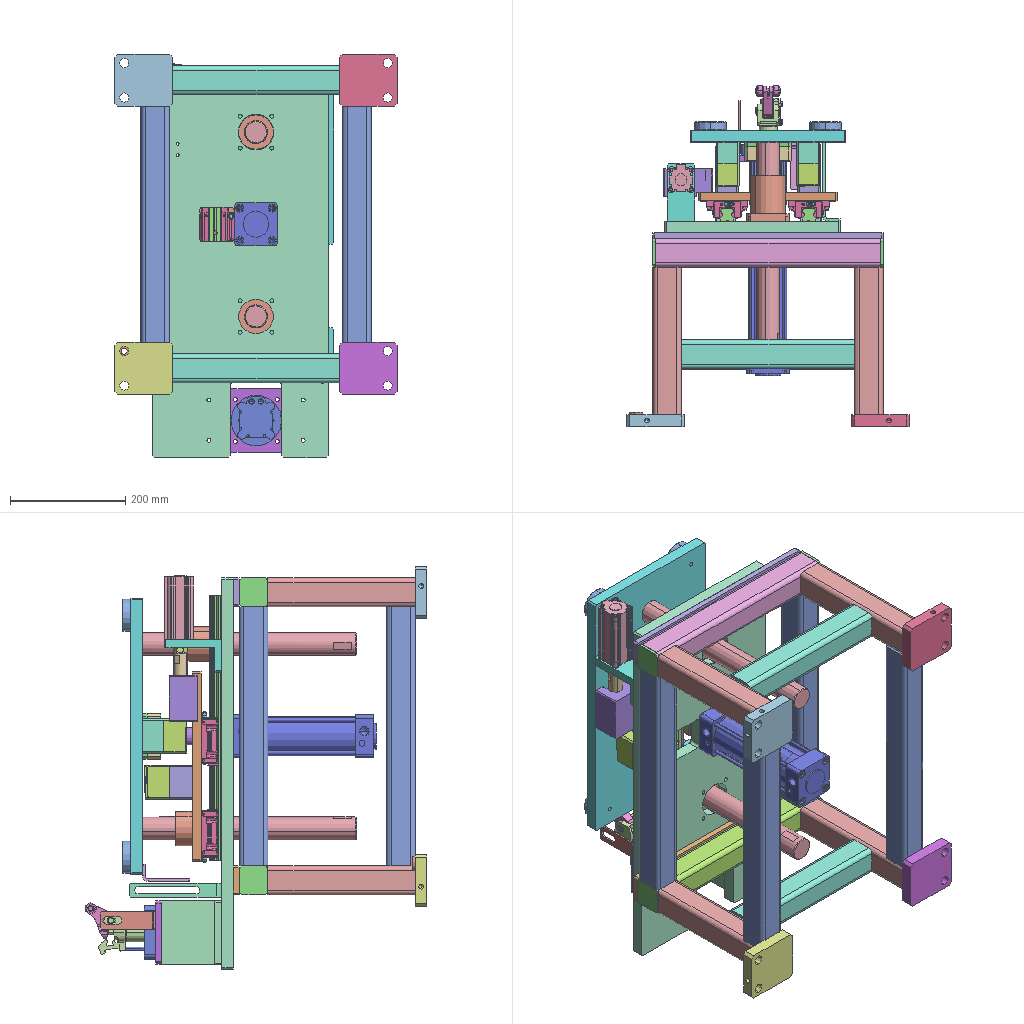Assembly | SolidWorks | 54 different items | 89 placed | box 490 x 593 x 700 mm
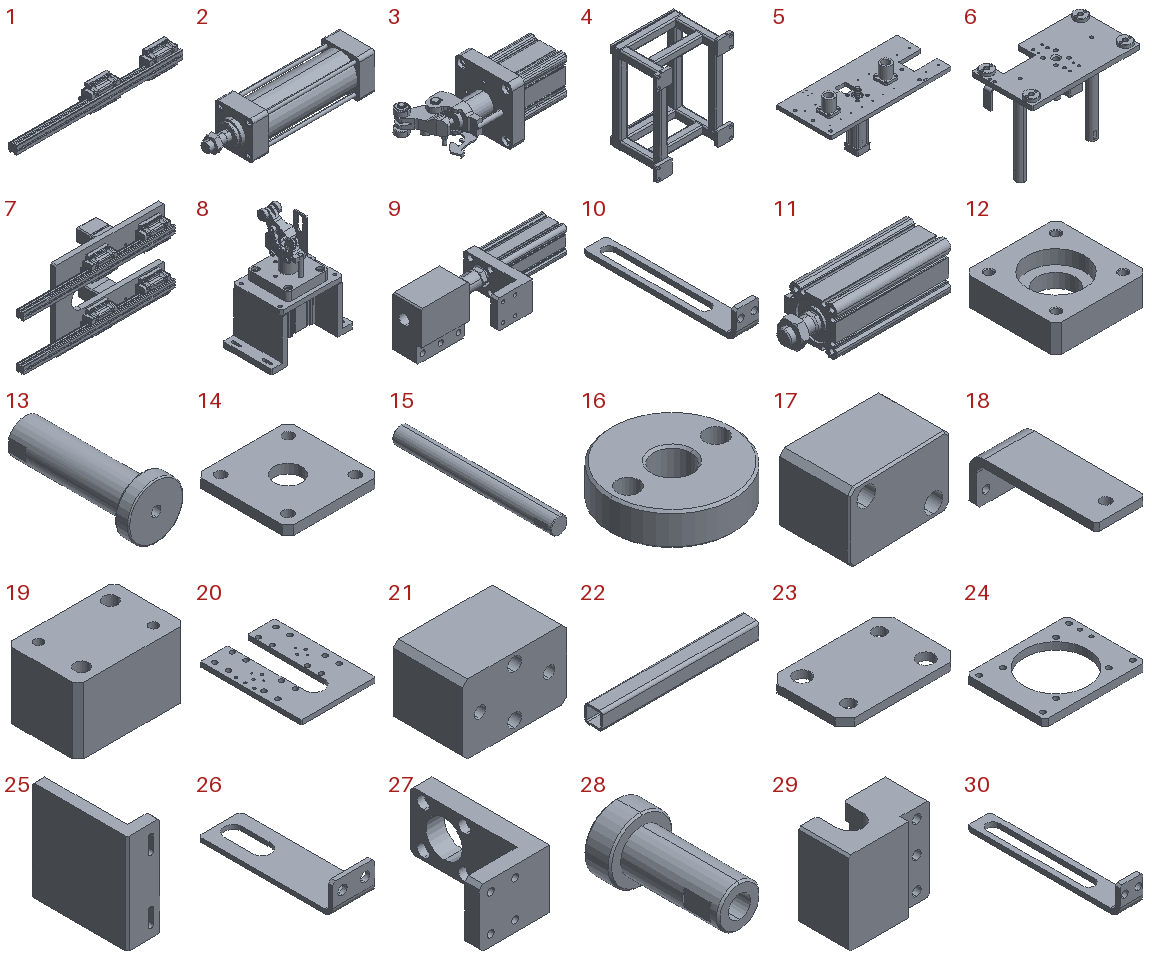Parts list (item | name | quantity | parent item | size | volume | features):
1 | (subassembly) | x2 | in 7 | 464.6 x 36 x 70 mm | 394256 mm3 | -
2 | (subassembly) | x1 | in 5 | 306 x 75 x 75 mm | 647112 mm3 | -
3 | (subassembly) | x1 | in 8 | 207.005 x 98.34 x 93 mm | 523956 mm3 | -
4 | (subassembly) | x1 | - | 490 x 336 x 590 mm | 4704318 mm3 | features HoleWzd 6
5 | (subassembly) | x1 | - | 680 x 305 x 348 mm | 4612161 mm3 | -
6 | (subassembly) | x1 | - | 492 x 270 x 407 mm | 3967388 mm3 | -
7 | (subassembly) | x1 | - | 464.6 x 134.966 x 242 mm | 2038560 mm3 | -
8 | (subassembly) | x1 | - | 184 x 110 x 237.505 mm | 955492 mm3 | features CompositeCurve 2
9 | (subassembly) | x1 | - | 253.005 x 100 x 85 mm | 494413 mm3 | -
10 | (subassembly) | x1 | - | 24 x 160 x 30 mm | 14225 mm3 | -
11 | (subassembly) | x1 | in 9 | 138.5 x 49.5 x 45 mm | 140577 mm3 | -
12 | - | x1 | in 6 | 80 x 80 x 24 mm | 116003 mm3 | features HoleWzd 2, Chamfer 1, Extrusion 1
13 | - | x1 | in 6 | 48 x 114 x 48 mm | 74222 mm3 | features HoleWzd 2, Fillet 1, ICE 1, Revolution 1
14 | - | x1 | in 6 | 80 x 80 x 8 mm | 45145 mm3 | features Chamfer 1, Extrusion 1
15 | - | x2 | in 6 | 40 x 380 x 40 mm | 474700 mm3 | features Chamfer 1, HoleWzd 1, ICE 1, Revolution 1
16 | - | x4 | in 6 | 56 x 56 x 15 mm | 31831 mm3 | features HoleWzd 2, Chamfer 1, Extrusion 1
17 | - | x4 | in 6, 7 | 60 x 39.966 x 40 mm | 86382 mm3 | features HoleWzd 3, Chamfer 2, Extrusion 1
18 | - | x1 | in 6 | 32 x 82 x 30 mm | 16187 mm3 | features HoleWzd 2, Chamfer 1, EdgeFlange 1, FlatPattern 1, SMBaseFlange 1, SheetMetal 1
19 | - | x2 | in 6 | 60 x 40 x 37 mm | 85137 mm3 | features HoleWzd 4, Chamfer 1, Extrusion 1
20 | - | x1 | in 7 | 242 x 330 x 15 mm | 894484 mm3 | features HoleWzd 4, Chamfer 1, Extrusion 1
21 | - | x2 | in 7 | 60 x 40 x 40 mm | 87063 mm3 | features HoleWzd 4, Chamfer 1, Extrusion 1
22 | - | x4 | in 4 | 450 x 50 x 50 mm | 383754 mm3 | features WeldMemberFeat 1, WeldmentFeature 1
23 | - | x1 | in 7 | 60 x 40 x 4 mm | 8672 mm3 | features Chamfer 1, Extrusion 1
24 | - | x1 | in 8 | 140 x 110 x 10 mm | 89465 mm3 | features HoleWzd 2, Chamfer 1, Extrusion 1
25 | - | x2 | in 8 | 36 x 105 x 110 mm | 166694 mm3 | features Chamfer 1, Extrusion 1, HoleWzd 1, ICE 1
26 | - | x1 | in 8 | 30 x 95 x 22 mm | 8685 mm3 | features ICE 2, Chamfer 1, EdgeFlange 1, FlatPattern 1, SMBaseFlange 1, SheetMetal 1
27 | - | x1 | in 9 | 58 x 100 x 48 mm | 82065 mm3 | features ICE 2, Chamfer 1, Extrusion 1, HoleWzd 1
28 | - | x1 | in 9 | 36 x 70 x 36 mm | 37200 mm3 | features Chamfer 1, HoleWzd 1, ICE 1, Revolution 1
29 | - | x1 | in 9 | 85 x 48 x 80 mm | 234146 mm3 | features HoleWzd 2, ICE 2, Chamfer 1, Extrusion 1
30 | - | x1 | in 10 | 24 x 160 x 30 mm | 14225 mm3 | features ICE 2, Chamfer 1, EdgeFlange 1, FlatPattern 1, SMBaseFlange 1, SheetMetal 1
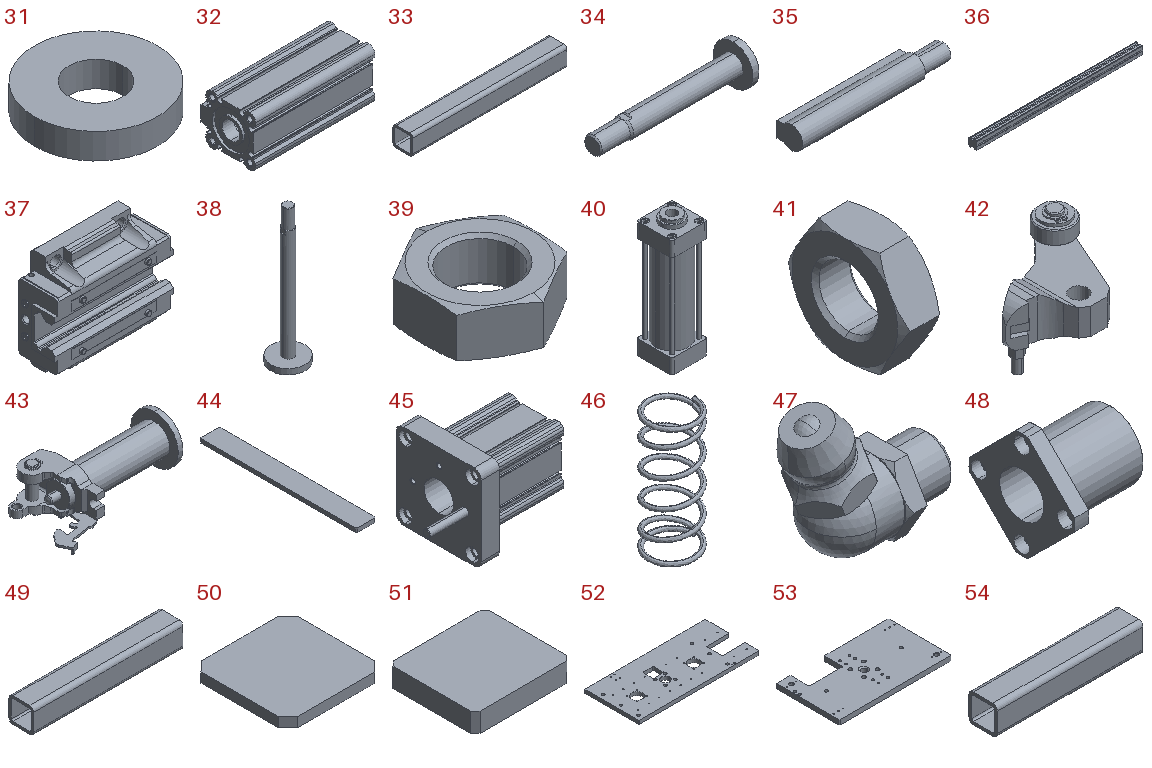31 | - | x1 | - | 24 x 24 x 5 mm | 1829 mm3 | features Extrusion 1
32 | - | x1 | in 11 | 110 x 49.5 x 45 mm | 111892 mm3 | features BaseBody 1
33 | - | x2 | in 4 | 390 x 50 x 50 mm | 332587 mm3 | features WeldMemberFeat 1, WeldmentFeature 1
34 | - | x1 | in 11 | 118.5 x 32 x 32 mm | 25635 mm3 | features BaseBody 1
35 | - | x2 | in 11 | 27 x 4.6 x 4 mm | 354.995 mm3 | features BaseBody 1
36 | - | x2 | in 1 | 460 x 22 x 23 mm | 189188 mm3 | features BaseBody 1
37 | - | x4 | in 1 | 83.1 x 30.5 x 70 mm | 101733 mm3 | features BaseBody 1
38 | - | x1 | in 2 | 63 x 63 x 249.5 mm | 104219 mm3 | features BaseBody 1
39 | - | x1 | in 2 | 27 x 31.177 x 11 mm | 4552 mm3 | features BaseBody 1
40 | - | x1 | in 2 | 75 x 75 x 262 mm | 538343 mm3 | features BaseBody 1
41 | - | x1 | in 11 | 8 x 25.403 x 22 mm | 2341 mm3 | features BaseBody 1
42 | - | x1 | in 3 | 64.335 x 54.505 x 46 mm | 29224 mm3 | features BaseBody 1
43 | - | x1 | in 3 | 135 x 70.758 x 50.5 mm | 116086 mm3 | features BaseBody 1
44 | - | x2 | in 4 | 50 x 400 x 10 mm | 199820 mm3 | features Chamfer 1, Extrusion 1
45 | - | x1 | in 3 | 146.5 x 93 x 93 mm | 378645 mm3 | features BaseBody 1
46 | - | x1 | in 9 | 16 x 16 x 40 mm | 423.431 mm3 | features BaseBody 1
47 | - | x4 | in 1 | 16.6 x 9.238 x 15.311 mm | 801.451 mm3 | features BaseBody 1
48 | - | x2 | in 5 | 80 x 96 x 96 mm | 154247 mm3 | features BaseBody 1
49 | - | x2 | in 4 | 300 x 50 x 50 mm | 255836 mm3 | features WeldMemberFeat 1, WeldmentFeature 1
50 | - | x4 | in 4 | 50 x 50 x 5 mm | 12250 mm3 | features Chamfer 1, Extrusion 1
51 | - | x4 | in 4 | 100 x 90 x 20 mm | 179000 mm3 | features Chamfer 1, Extrusion 1
52 | - | x1 | in 5 | 680 x 305 x 20 mm | 3656558 mm3 | features HoleWzd 7, Chamfer 2, Extrusion 1, Fillet 1, ICE 1
53 | - | x1 | in 6 | 480 x 270 x 20 mm | 2296067 mm3 | features HoleWzd 9, Chamfer 3, Extrusion 1, Fillet 1
54 | - | x4 | in 4 | 256 x 50 x 50 mm | 218314 mm3 | features WeldMemberFeat 1, WeldmentFeature 1
Mates (type | each side: item.copy, entity, surface, feature):
In the top assembly
Coincident | 44.1 face plane | 52.1 face plane Boss-Extrude1
Concentric | 44.2 face cylinder M8 Tapped Hole1 | 52.1 face cylinder Hole1 | 2 times
Concentric | 48.1 face cylinder Input1 | 15.1 face cylinder Revolve1
Concentric | 48.2 face cylinder Input1 | 15.2 face cylinder Revolve1
Coincident | 52.1 face plane Boss-Extrude1 | 25.1 face plane Boss-Extrude1
Tangent | 52.1 face cylinder M8 Tapped Hole1 | 25.1 face plane Cut-Extrude1 | 2 times
Coincident | 52.1 face plane Boss-Extrude1 | 36.1 face plane Input1
Concentric | 52.1 face cylinder M6 Tapped Hole2 | 36.1 face cylinder Input1
Concentric | 52.1 face cylinder M6 Tapped Hole2 | 36.2 face cylinder Input1
Concentric | 52.1 face cylinder M6 Tapped Hole3 | 27.1 face cylinder Cut-Extrude2 | 2 times
Coincident | 52.1 face plane Boss-Extrude1 | 27.1 face plane Boss-Extrude1
Concentric | 52.1 face cylinder M6 Tapped Hole1 | 30.1 face cylinder Cut-Extrude2 | 2 times
Coincident | 52.1 face plane Boss-Extrude1 | 30.1 face plane Edge-Flange1
Coincident | 51.1 face plane | 31.1 face plane Boss-Extrude1
Concentric | 51.1 face cylinder Hole2 | 31.1 face cylinder Boss-Extrude1
In subassembly 6
Concentric | 53.1 face cylinder Hole7 | 12.1 face cylinder Hole1
Concentric | 53.1 face cylinder Hole4 | 12.1 face cylinder M8 Tapped Hole1
Coincident | 12.1 face plane Hole1 | 13.1 face plane Revolve1
Concentric | 53.1 face cylinder Hole7 | 13.1 face cylinder Revolve1
Concentric | 53.1 face cylinder Hole7 | 14.1 face cylinder Boss-Extrude1
Concentric | 53.1 face cylinder Hole4 | 14.1 face cylinder Boss-Extrude1
Coincident | 12.1 face plane Boss-Extrude1 | 14.1 face plane Boss-Extrude1
Coincident | 53.1 face plane Boss-Extrude1 | 14.1 face plane Boss-Extrude1
Concentric | 53.1 face cylinder Hole8 | 15.3 face cylinder Revolve1
Concentric | 53.1 face cylinder Hole8 | 15.4 face cylinder Revolve1
Coincident | 53.1 face plane Hole8 | 15.3 face plane Revolve1
Coincident | 53.1 face plane Hole8 | 15.4 face plane Revolve1
Concentric | 53.1 face cylinder Hole3 | 16.1 face cylinder Hole1
Coincident | 53.1 face plane Boss-Extrude1 | 16.1 face plane Boss-Extrude1
Concentric | 53.1 face cylinder M5 Tapped Hole1 | 16.1 face cylinder Hole2
Coincident | 53.1 face plane Boss-Extrude1 | 16.2 face plane Boss-Extrude1
Concentric | 53.1 face cylinder M8x1.0 Tapped Hole1 | 16.2 face cylinder Hole1
Concentric | 53.1 face cylinder M5 Tapped Hole1 | 16.2 face cylinder Hole2
Coincident | 53.1 face plane Boss-Extrude1 | 16.3 face plane Boss-Extrude1
Concentric | 53.1 face cylinder M8x1.0 Tapped Hole1 | 16.3 face cylinder Hole1
Concentric | 53.1 face cylinder M5 Tapped Hole1 | 16.3 face cylinder Hole2
Concentric | 53.1 face cylinder Hole3 | 16.4 face cylinder Hole1
Concentric | 53.1 face cylinder M5 Tapped Hole1 | 16.4 face cylinder Hole2
Coincident | 53.1 face plane Boss-Extrude1 | 16.4 face plane Boss-Extrude1
Coincident | 19.1 face plane Boss-Extrude1 | 19.2 face plane Boss-Extrude1
Coincident | 53.1 face plane Boss-Extrude1 | 19.1 face plane Boss-Extrude1
Lock | 53.1 select_type:0 | 19.1 select_type:0
Lock | 53.1 select_type:0 | 19.2 select_type:0
Concentric | 17.1 face cylinder Hole2 | 19.1 face cylinder M6 Tapped Hole2
Coincident | 17.1 face plane Boss-Extrude1 | 19.1 face plane Boss-Extrude1 | 2 times
Coincident | 17.2 face plane Boss-Extrude1 | 19.2 face plane Boss-Extrude1 | 3 times
Coincident | 53.1 face plane Boss-Extrude1 | 18.1 face plane Edge-Flange1
Concentric | 53.1 face cylinder Hole2 | 18.1 face cylinder M6 Tapped Hole1 | 2 times
In subassembly 5
Concentric | 52.2 face cylinder M8 Tapped Hole2 | 48.3 face cylinder Input1
Coincident | 52.2 face plane Boss-Extrude1 | 48.3 face plane Input1
Parallel | 52.2 face plane Boss-Extrude1 | 48.3 face plane Input1
Coincident | 52.2 face plane Boss-Extrude1 | 48.4 face plane Input1
Concentric | 52.2 face cylinder M8 Tapped Hole2 | 48.4 face cylinder Input1
Parallel | 52.2 face plane Boss-Extrude1 | 48.4 face plane Input1
Coincident | 52.2 face plane Boss-Extrude1 | 40.1 face plane Input1
Concentric | 52.2 face cylinder Cut-Extrude1 | 38.1 face cylinder Input1
Parallel | 52.2 face plane Boss-Extrude1 | 40.1 face plane Input1
In subassembly 9
Concentric | 27.2 face cylinder Cut-Extrude1 | 28.1 face cylinder Revolve1
Coincident | 28.1 face plane Revolve1 | 29.1 face plane Cut-Extrude2
Concentric | 28.1 face cylinder Revolve1 | 29.1 face cylinder Cut-Extrude1
Parallel | 27.2 face plane Boss-Extrude1 | 29.1 face plane Boss-Extrude1
Tangent | 29.1 face cylinder M20 Tapped Hole1 | 46.1 face surface:4006 Input1
Lock | 28.1 select_type:0 | 46.1 select_type:0
Concentric | 27.2 face cylinder Cut-Extrude1 | 34.1 face cylinder Input1
Concentric | 27.2 face cylinder Hole size (per) hex socket cap screw type 1 | 32.1 face cylinder Input1
Coincident | 27.2 face plane Boss-Extrude1 | 32.1 face plane Input1
Concentric | 28.1 face cylinder M14x1.5 Tapped Hole1 | 34.1 face cylinder Input1
In subassembly 8
Concentric | 24.1 face cylinder M6 Tapped Hole1 | 26.1 face cylinder Cut-Extrude2 | 2 times
Coincident | 24.1 face plane Boss-Extrude1 | 26.1 face plane Edge-Flange1
Concentric | 24.1 face cylinder Boss-Extrude1 | 25.2 face cylinder M6 Tapped Hole1 | 2 times
Coincident | 24.1 face plane Boss-Extrude1 | 25.2 face plane Boss-Extrude1
Concentric | 24.1 edge | 25.3 edge
Concentric | 24.1 face cylinder Boss-Extrude1 | 25.3 face cylinder M6 Tapped Hole1
Coincident | 24.1 face plane Boss-Extrude1 | 25.3 face plane Boss-Extrude1
Concentric | 24.1 face cylinder M8 Tapped Hole1 | 45.1 face cylinder Input1 | 2 times
Coincident | 24.1 face plane Boss-Extrude1 | 45.1 face plane Input1
In subassembly 7
Concentric | 20.1 face cylinder M6 Tapped Hole1 | 21.1 face cylinder Hole1 | 2 times
Coincident | 20.1 face plane Boss-Extrude1 | 21.1 face plane Boss-Extrude1
Concentric | 20.1 face cylinder M6 Tapped Hole1 | 21.2 face cylinder Hole1
Coincident | 20.1 face plane Boss-Extrude1 | 21.2 face plane Boss-Extrude1
Parallel | 21.1 face plane Boss-Extrude1 | 21.2 face plane Boss-Extrude1
Coincident | 37.1 face plane Input1 | 37.2 face plane Input1
Coincident | 20.1 face plane Boss-Extrude1 | 37.1 face plane Input1
Parallel | 20.1 face plane Boss-Extrude1 | 37.1 face plane Input1
Coincident | 21.1 face plane Boss-Extrude1 | 23.1 face plane Boss-Extrude1
Concentric | 21.1 face cylinder Hole2 | 23.1 face cylinder Boss-Extrude1 | 2 times
Coincident | 21.2 face plane Boss-Extrude1 | 17.1 face plane Boss-Extrude1 | 3 times
Coincident | 17.1 face plane Boss-Extrude1 | 17.2 face plane Boss-Extrude1
Coincident | 21.1 face plane Boss-Extrude1 | 17.2 face plane Boss-Extrude1
Coincident | 23.1 face plane Boss-Extrude1 | 17.2 face plane Boss-Extrude1
Concentric | 20.1 face cylinder Hole1 | 37.3 face cylinder Input1
Concentric | 20.1 face cylinder Hole1 | 37.4 face cylinder Input1
In subassembly 1
DistanceDim | 37.5 face plane Input1 | 36.3 face plane Input1 | 3 times
DistanceDim | 37.6 face plane Input1 | 36.3 face plane Input1 | 2 times
Concentric | 37.6 face cylinder Input1 | 47.1 face cylinder Input1
Coincident | 37.6 face plane Input1 | 47.1 face plane Input1
Concentric | 37.5 face cylinder Input1 | 47.2 face cylinder Input1
Coincident | 37.5 face plane Input1 | 47.2 face plane Input1
DistanceDim | 37.5 face plane Input1 | 37.6 face plane Input1
In subassembly 4
Coincident | 54.1 face plane Cold-formed square hollow section GB/T 6728-2002 50 X 50 X 4(1) | 54.2 face plane Cold-formed square hollow section GB/T 6728-2002 50 X 50 X 4(1)
Coincident | 54.1 face plane Cold-formed square hollow section GB/T 6728-2002 50 X 50 X 4(1) | 54.3 face plane Cold-formed square hollow section GB/T 6728-2002 50 X 50 X 4(1)
Coincident | 54.1 face plane Cold-formed square hollow section GB/T 6728-2002 50 X 50 X 4(1) | 54.4 face plane Cold-formed square hollow section GB/T 6728-2002 50 X 50 X 4(1)
Coincident | 54.2 face plane Cold-formed square hollow section GB/T 6728-2002 50 X 50 X 4(1) | 22.1 face plane Cold-formed square hollow section GB/T 6728-2002 50 X 50 X 4(1) | 3 times
Coincident | 54.1 face plane Cold-formed square hollow section GB/T 6728-2002 50 X 50 X 4(1) | 22.1 face plane Cold-formed square hollow section GB/T 6728-2002 50 X 50 X 4(1) | 2 times
Coincident | 54.2 face plane Cold-formed square hollow section GB/T 6728-2002 50 X 50 X 4(1) | 22.2 face plane Cold-formed square hollow section GB/T 6728-2002 50 X 50 X 4(1) | 3 times
Coincident | 54.4 face plane Cold-formed square hollow section GB/T 6728-2002 50 X 50 X 4(1) | 22.3 face plane Cold-formed square hollow section GB/T 6728-2002 50 X 50 X 4(1) | 3 times
Coincident | 22.3 face plane Cold-formed square hollow section GB/T 6728-2002 50 X 50 X 4(1) | 22.4 face plane Cold-formed square hollow section GB/T 6728-2002 50 X 50 X 4(1)
Coincident | 54.4 face plane Cold-formed square hollow section GB/T 6728-2002 50 X 50 X 4(1) | 22.4 face plane Cold-formed square hollow section GB/T 6728-2002 50 X 50 X 4(1) | 3 times
Coincident | 54.3 face plane Cold-formed square hollow section GB/T 6728-2002 50 X 50 X 4(1) | 22.3 face plane Cold-formed square hollow section GB/T 6728-2002 50 X 50 X 4(1) | 2 times
Coincident | 54.2 face plane Cold-formed square hollow section GB/T 6728-2002 50 X 50 X 4(1) | 54.3 face plane Cold-formed square hollow section GB/T 6728-2002 50 X 50 X 4(1)
Coincident | 54.4 face plane Cold-formed square hollow section GB/T 6728-2002 50 X 50 X 4(1) | 33.1 face plane
Coincident | 22.4 face plane Cold-formed square hollow section GB/T 6728-2002 50 X 50 X 4(1) | 33.1 face plane
Coincident | 54.3 face plane Cold-formed square hollow section GB/T 6728-2002 50 X 50 X 4(1) | 33.2 face plane | 2 times
Coincident | 54.4 face plane Cold-formed square hollow section GB/T 6728-2002 50 X 50 X 4(1) | 49.1 face plane Cold-formed square hollow section GB/T 6728-2002 50 X 50 X 4(1) | 2 times
Coincident | 54.3 face plane Cold-formed square hollow section GB/T 6728-2002 50 X 50 X 4(1) | 49.2 face plane Cold-formed square hollow section GB/T 6728-2002 50 X 50 X 4(1)
Coincident | 54.2 face plane Cold-formed square hollow section GB/T 6728-2002 50 X 50 X 4(1) | 49.2 face plane Cold-formed square hollow section GB/T 6728-2002 50 X 50 X 4(1)
Coincident | 33.1 face plane | 44.3 face plane | 2 times
Coincident | 54.1 face plane Cold-formed square hollow section GB/T 6728-2002 50 X 50 X 4(1) | 49.1 face plane Cold-formed square hollow section GB/T 6728-2002 50 X 50 X 4(1)
Coincident | 33.2 face plane | 50.1 face plane Boss-Extrude1 | 3 times
Coincident | 54.3 face plane Cold-formed square hollow section GB/T 6728-2002 50 X 50 X 4(1) | 50.1 face plane Boss-Extrude1
Coincident | 33.1 face plane | 50.2 face plane Boss-Extrude1 | 3 times
Coincident | 33.1 face plane | 50.3 face plane Boss-Extrude1 | 3 times
Coincident | 33.2 face plane | 50.4 face plane Boss-Extrude1 | 3 times
Coincident | 44.3 face plane | 50.3 face plane Boss-Extrude1
Coincident | 33.2 face plane | 44.4 face plane | 2 times
Coincident | 44.4 face plane | 50.4 face plane Boss-Extrude1
Coincident | 54.2 face plane Cold-formed square hollow section GB/T 6728-2002 50 X 50 X 4(1) | 51.2 face plane
Coincident | 54.1 face plane Cold-formed square hollow section GB/T 6728-2002 50 X 50 X 4(1) | 51.3 face plane
Coincident | 54.3 face plane Cold-formed square hollow section GB/T 6728-2002 50 X 50 X 4(1) | 51.4 face plane
Coincident | 54.4 face plane Cold-formed square hollow section GB/T 6728-2002 50 X 50 X 4(1) | 51.5 face plane
Coincident | 51.2 face plane | 51.4 face plane
DistanceDim | 51.4 face plane | 51.2 face plane
Parallel | 54.3 face plane Cold-formed square hollow section GB/T 6728-2002 50 X 50 X 4(1) | 51.4 face plane
Coincident | 51.5 face plane | 51.3 face plane
DistanceDim | 51.3 face plane | 51.5 face plane
Parallel | 54.1 face plane Cold-formed square hollow section GB/T 6728-2002 50 X 50 X 4(1) | 51.3 face plane
DistanceDim | 51.2 face plane | 51.3 face plane
DistanceDim | 51.2 face plane | 54.2 face plane Cold-formed square hollow section GB/T 6728-2002 50 X 50 X 4(1) | 2 times
Coincident | 51.2 face plane | 51.3 face plane | 2 times
Coincident | 49.1 face plane Cold-formed square hollow section GB/T 6728-2002 50 X 50 X 4(1) | 49.2 face plane Cold-formed square hollow section GB/T 6728-2002 50 X 50 X 4(1)
DistanceDim | 49.1 face plane Cold-formed square hollow section GB/T 6728-2002 50 X 50 X 4(1) | 51.3 face plane